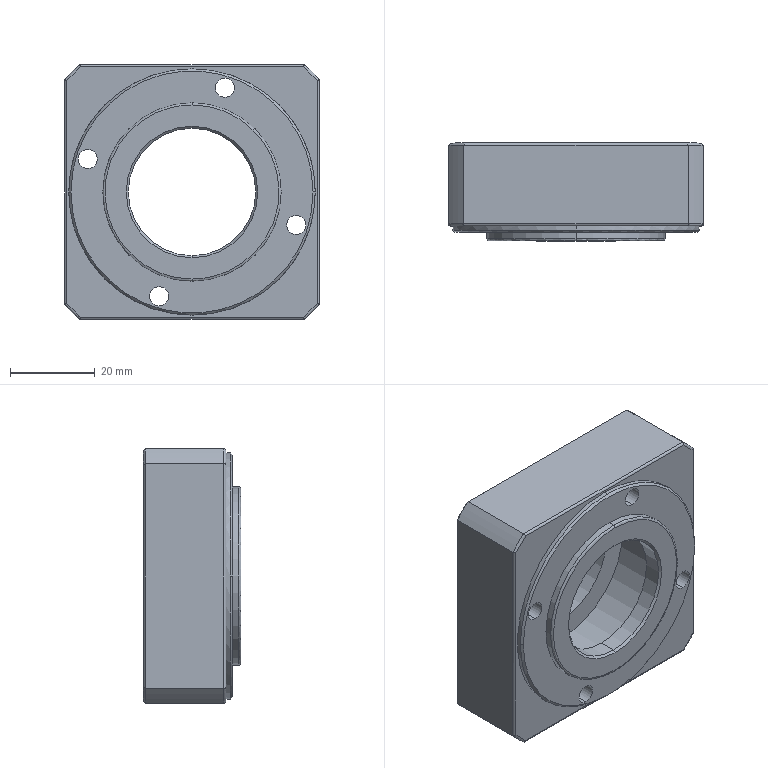Part | STEP file | _X2_8f9351656cd55170_X0_MAB060-30-46-M4 | 1 solid | 102 faces | box 60 x 23 x 60 mm | volume 47434 mm3 | cylinder 44 | cone 34 | plane 18 | spline 6 | commonest cylinder face diameters 3.3 x8 4.5 x8 7.5 x8 1 x4 30 x4 80 x4